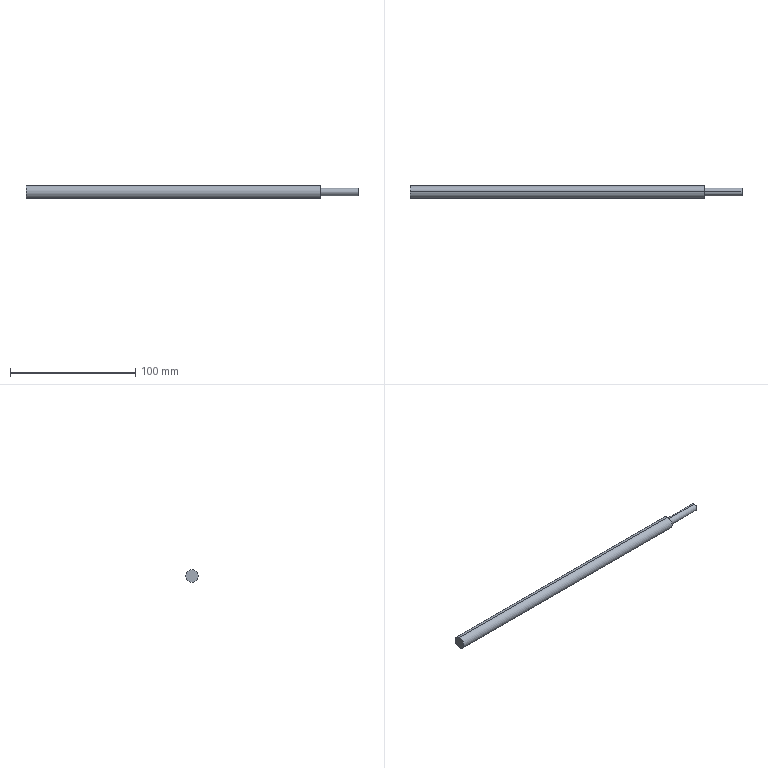Part | SolidWorks | features BaseBody 1, ICE 1 | 1 solid | 7 faces | box 264.77 x 10 x 10 mm | volume 19287 mm3 | cylinder 4 | plane 3 | commonest cylinder face diameters 6 x2 10 x2
STEP:
#1=CARTESIAN_POINT('',(0.,0.,-5.));
#2=VERTEX_POINT('',#1);
#3=CARTESIAN_POINT('',(0.,0.,5.));
#4=VERTEX_POINT('',#3);
#5=CARTESIAN_POINT('',(0.,0.,0.));
#6=DIRECTION('',(1.,0.,0.));
#7=DIRECTION('',(0.,0.,-1.));
#8=AXIS2_PLACEMENT_3D('',#5,#6,#7);
#9=CIRCLE('',#8,5.);
#10=EDGE_CURVE('',#2,#4,#9,.T.);
#11=ORIENTED_EDGE('',*,*,#10,.T.);
#12=CARTESIAN_POINT('',(234.77,0.,5.));
#13=VERTEX_POINT('',#12);
#14=CARTESIAN_POINT('',(-0.23,0.,5.));
#15=DIRECTION('',(1.,0.,0.));
#16=VECTOR('',#15,1000.);
#17=LINE('',#14,#16);
#18=EDGE_CURVE('',#4,#13,#17,.T.);
#19=ORIENTED_EDGE('',*,*,#18,.T.);
#20=CARTESIAN_POINT('',(234.77,0.,-5.));
#21=VERTEX_POINT('',#20);
#22=CARTESIAN_POINT('',(234.77,0.,0.));
#23=DIRECTION('',(1.,0.,0.));
#24=DIRECTION('',(0.,0.,-1.));
#25=AXIS2_PLACEMENT_3D('',#22,#23,#24);
#26=CIRCLE('',#25,5.);
#27=EDGE_CURVE('',#21,#13,#26,.T.);
#28=ORIENTED_EDGE('',*,*,#27,.F.);
#29=CARTESIAN_POINT('',(-0.23,0.,-5.));
#30=DIRECTION('',(1.,0.,0.));
#31=VECTOR('',#30,1000.);
#32=LINE('',#29,#31);
#33=EDGE_CURVE('',#2,#21,#32,.T.);
#34=ORIENTED_EDGE('',*,*,#33,.F.);
#35=EDGE_LOOP('',(#11,#19,#28,#34));
#36=FACE_OUTER_BOUND('',#35,.T.);
#37=CARTESIAN_POINT('',(-0.23,0.,0.));
#38=DIRECTION('',(1.,0.,0.));
#39=DIRECTION('',(0.,0.,-1.));
#40=AXIS2_PLACEMENT_3D('',#37,#38,#39);
#41=CYLINDRICAL_SURFACE('',#40,5.);
#42=ADVANCED_FACE('',(#36),#41,.T.);
#43=CARTESIAN_POINT('',(264.77,0.,-3.));
#44=VERTEX_POINT('',#43);
#45=CARTESIAN_POINT('',(264.77,0.,3.));
#46=VERTEX_POINT('',#45);
#47=CARTESIAN_POINT('',(264.77,0.,0.));
#48=DIRECTION('',(1.,0.,0.));
#49=DIRECTION('',(0.,0.,-1.));
#50=AXIS2_PLACEMENT_3D('',#47,#48,#49);
#51=CIRCLE('',#50,3.);
#52=EDGE_CURVE('',#44,#46,#51,.T.);
#53=ORIENTED_EDGE('',*,*,#52,.F.);
#54=CARTESIAN_POINT('',(234.77,0.,-3.));
#55=VERTEX_POINT('',#54);
#56=CARTESIAN_POINT('',(264.77,0.,-3.));
#57=DIRECTION('',(-1.,0.,0.));
#58=VECTOR('',#57,1000.);
#59=LINE('',#56,#58);
#60=EDGE_CURVE('',#44,#55,#59,.T.);
#61=ORIENTED_EDGE('',*,*,#60,.T.);
#62=CARTESIAN_POINT('',(234.77,0.,3.));
#63=VERTEX_POINT('',#62);
#64=CARTESIAN_POINT('',(234.77,0.,0.));
#65=DIRECTION('',(1.,0.,0.));
#66=DIRECTION('',(0.,0.,-1.));
#67=AXIS2_PLACEMENT_3D('',#64,#65,#66);
#68=CIRCLE('',#67,3.);
#69=EDGE_CURVE('',#55,#63,#68,.T.);
#70=ORIENTED_EDGE('',*,*,#69,.T.);
#71=CARTESIAN_POINT('',(264.77,0.,3.));
#72=DIRECTION('',(-1.,0.,0.));
#73=VECTOR('',#72,1000.);
#74=LINE('',#71,#73);
#75=EDGE_CURVE('',#46,#63,#74,.T.);
#76=ORIENTED_EDGE('',*,*,#75,.F.);
#77=EDGE_LOOP('',(#53,#61,#70,#76));
#78=FACE_OUTER_BOUND('',#77,.T.);
#79=CARTESIAN_POINT('',(264.77,0.,0.));
#80=DIRECTION('',(-1.,0.,0.));
#81=DIRECTION('',(0.,0.,1.));
#82=AXIS2_PLACEMENT_3D('',#79,#80,#81);
#83=CYLINDRICAL_SURFACE('',#82,3.);
#84=ADVANCED_FACE('',(#78),#83,.T.);
#85=CARTESIAN_POINT('',(234.77,0.,0.));
#86=DIRECTION('',(1.,0.,0.));
#87=DIRECTION('',(0.,0.,-1.));
#88=AXIS2_PLACEMENT_3D('',#85,#86,#87);
#89=CIRCLE('',#88,3.);
#90=EDGE_CURVE('',#63,#55,#89,.T.);
#91=ORIENTED_EDGE('',*,*,#90,.F.);
#92=ORIENTED_EDGE('',*,*,#69,.F.);
#93=EDGE_LOOP('',(#91,#92));
#94=FACE_BOUND('',#93,.T.);
#95=ORIENTED_EDGE('',*,*,#27,.T.);
#96=CARTESIAN_POINT('',(234.77,0.,0.));
#97=DIRECTION('',(1.,0.,0.));
#98=DIRECTION('',(0.,0.,-1.));
#99=AXIS2_PLACEMENT_3D('',#96,#97,#98);
#100=CIRCLE('',#99,5.);
#101=EDGE_CURVE('',#13,#21,#100,.T.);
#102=ORIENTED_EDGE('',*,*,#101,.T.);
#103=EDGE_LOOP('',(#95,#102));
#104=FACE_OUTER_BOUND('',#103,.T.);
#105=CARTESIAN_POINT('',(234.77,0.,0.));
#106=DIRECTION('',(1.,0.,0.));
#107=DIRECTION('',(0.,0.,-1.));
#108=AXIS2_PLACEMENT_3D('',#105,#106,#107);
#109=PLANE('',#108);
#110=ADVANCED_FACE('',(#94,#104),#109,.T.);
#111=ORIENTED_EDGE('',*,*,#60,.F.);
#112=CARTESIAN_POINT('',(264.77,0.,0.));
#113=DIRECTION('',(1.,0.,0.));
#114=DIRECTION('',(0.,0.,-1.));
#115=AXIS2_PLACEMENT_3D('',#112,#113,#114);
#116=CIRCLE('',#115,3.);
#117=EDGE_CURVE('',#46,#44,#116,.T.);
#118=ORIENTED_EDGE('',*,*,#117,.F.);
#119=ORIENTED_EDGE('',*,*,#75,.T.);
#120=ORIENTED_EDGE('',*,*,#90,.T.);
#121=EDGE_LOOP('',(#111,#118,#119,#120));
#122=FACE_OUTER_BOUND('',#121,.T.);
#123=CARTESIAN_POINT('',(264.77,0.,0.));
#124=DIRECTION('',(-1.,0.,0.));
#125=DIRECTION('',(0.,0.,1.));
#126=AXIS2_PLACEMENT_3D('',#123,#124,#125);
#127=CYLINDRICAL_SURFACE('',#126,3.);
#128=ADVANCED_FACE('',(#122),#127,.T.);
#129=ORIENTED_EDGE('',*,*,#117,.T.);
#130=ORIENTED_EDGE('',*,*,#52,.T.);
#131=EDGE_LOOP('',(#129,#130));
#132=FACE_OUTER_BOUND('',#131,.T.);
#133=CARTESIAN_POINT('',(264.77,0.,0.));
#134=DIRECTION('',(1.,0.,0.));
#135=DIRECTION('',(0.,0.,-1.));
#136=AXIS2_PLACEMENT_3D('',#133,#134,#135);
#137=PLANE('',#136);
#138=ADVANCED_FACE('',(#132),#137,.T.);
#139=ORIENTED_EDGE('',*,*,#18,.F.);
#140=CARTESIAN_POINT('',(0.,0.,0.));
#141=DIRECTION('',(1.,0.,0.));
#142=DIRECTION('',(0.,0.,-1.));
#143=AXIS2_PLACEMENT_3D('',#140,#141,#142);
#144=CIRCLE('',#143,5.);
#145=EDGE_CURVE('',#4,#2,#144,.T.);
#146=ORIENTED_EDGE('',*,*,#145,.T.);
#147=ORIENTED_EDGE('',*,*,#33,.T.);
#148=ORIENTED_EDGE('',*,*,#101,.F.);
#149=EDGE_LOOP('',(#139,#146,#147,#148));
#150=FACE_OUTER_BOUND('',#149,.T.);
#151=CARTESIAN_POINT('',(-0.23,0.,0.));
#152=DIRECTION('',(1.,0.,0.));
#153=DIRECTION('',(0.,0.,-1.));
#154=AXIS2_PLACEMENT_3D('',#151,#152,#153);
#155=CYLINDRICAL_SURFACE('',#154,5.);
#156=ADVANCED_FACE('',(#150),#155,.T.);
#157=ORIENTED_EDGE('',*,*,#10,.F.);
#158=ORIENTED_EDGE('',*,*,#145,.F.);
#159=EDGE_LOOP('',(#157,#158));
#160=FACE_OUTER_BOUND('',#159,.T.);
#161=CARTESIAN_POINT('',(0.,0.,0.));
#162=DIRECTION('',(1.,0.,0.));
#163=DIRECTION('',(0.,0.,-1.));
#164=AXIS2_PLACEMENT_3D('',#161,#162,#163);
#165=PLANE('',#164);
#166=ADVANCED_FACE('',(#160),#165,.F.);
#167=CLOSED_SHELL('',(#42,#84,#110,#128,#138,#156,#166));
#168=MANIFOLD_SOLID_BREP('',#167);
#169=CARTESIAN_POINT('',(0.,0.,0.));
#170=DIRECTION('',(0.,0.,1.));
#171=DIRECTION('',(1.,0.,0.));
#172=AXIS2_PLACEMENT_3D('',#169,#170,#171);
#173=(LENGTH_UNIT()NAMED_UNIT(*)SI_UNIT(.MILLI.,.METRE.));
#174=UNCERTAINTY_MEASURE_WITH_UNIT(LENGTH_MEASURE(0.00001),#173,'','');
#175=(NAMED_UNIT(*)PLANE_ANGLE_UNIT()SI_UNIT($,.RADIAN.));
#176=(NAMED_UNIT(*)SI_UNIT($,.STERADIAN.)SOLID_ANGLE_UNIT());
#177=(GEOMETRIC_REPRESENTATION_CONTEXT(3)GLOBAL_UNCERTAINTY_ASSIGNED_CONTEXT((#174))GLOBAL_UNIT_ASSIGNED_CONTEXT((#173,#175,#176))REPRESENTATION_CONTEXT('',''));
#178=ADVANCED_BREP_SHAPE_REPRESENTATION('',(#168,#172),#177);